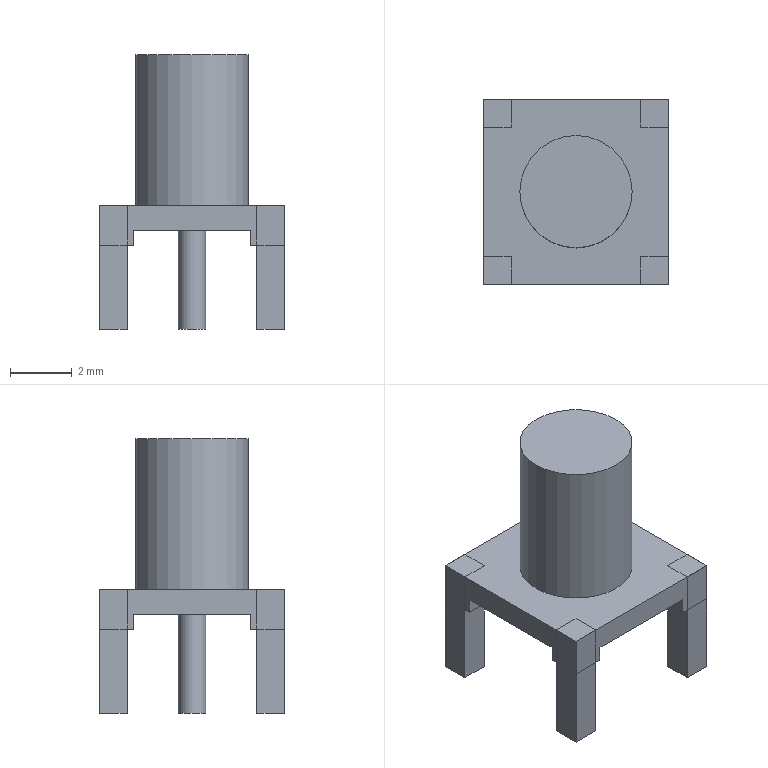Part | STEP file | MCX-JHD | 7 solids | 48 faces | box 6 x 6 x 8.9 mm | volume 97.715 mm3 | plane 46 | cylinder 2 | commonest cylinder face diameters 0.9 x1 3.64 x1